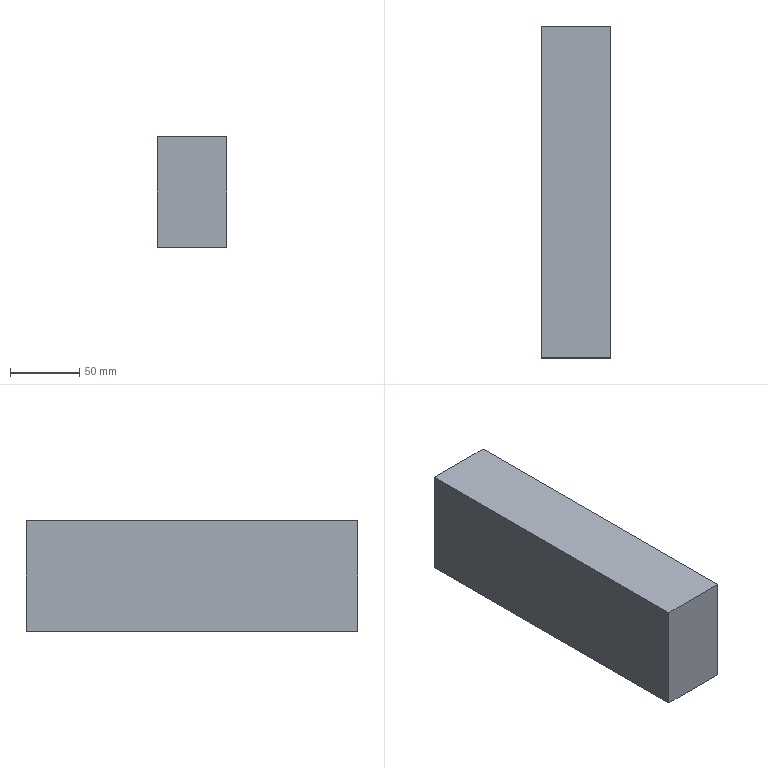Part | STEP file | Tube necking machine_id542_x_t | 1 solid | 6 faces | box 50 x 240 x 80 mm | volume 960000 mm3 | plane 6
STEP:
#1=CARTESIAN_POINT('',(0.,0.,0.));
#2=DIRECTION('',(0.,0.,1.));
#3=DIRECTION('',(1.,0.,0.));
#4=AXIS2_PLACEMENT_3D('',#1,#2,#3);
#5=CARTESIAN_POINT('',(160.,220.,0.));
#6=VERTEX_POINT('',#5);
#7=CARTESIAN_POINT('',(160.,-20.,0.));
#8=VERTEX_POINT('',#7);
#9=CARTESIAN_POINT('',(160.,220.,0.));
#10=DIRECTION('',(0.,-1.,0.));
#11=VECTOR('',#10,1.);
#12=LINE('',#9,#11);
#13=CARTESIAN_POINT('',(160.,220.,80.));
#14=DIRECTION('',(1.,0.,0.));
#15=DIRECTION('',(0.,1.,0.));
#16=AXIS2_PLACEMENT_3D('',#13,#14,#15);
#17=PLANE('',#16);
#18=CARTESIAN_POINT('',(0.,-80.));
#19=DIRECTION('',(-1.,0.));
#20=VECTOR('',#19,1.);
#21=LINE('',#18,#20);
#22=(GEOMETRIC_REPRESENTATION_CONTEXT(2)PARAMETRIC_REPRESENTATION_CONTEXT()REPRESENTATION_CONTEXT('',''));
#23=DEFINITIONAL_REPRESENTATION('',(#21),#22);
#24=PCURVE('',#17,#23);
#25=CARTESIAN_POINT('',(0.,0.,0.));
#26=DIRECTION('',(0.,0.,1.));
#27=DIRECTION('',(1.,0.,0.));
#28=AXIS2_PLACEMENT_3D('',#25,#26,#27);
#29=PLANE('',#28);
#30=CARTESIAN_POINT('',(160.,220.));
#31=DIRECTION('',(0.,-1.));
#32=VECTOR('',#31,1.);
#33=LINE('',#30,#32);
#34=(GEOMETRIC_REPRESENTATION_CONTEXT(2)PARAMETRIC_REPRESENTATION_CONTEXT()REPRESENTATION_CONTEXT('',''));
#35=DEFINITIONAL_REPRESENTATION('',(#33),#34);
#36=PCURVE('',#29,#35);
#37=SURFACE_CURVE('',#12,(#24,#36),.PCURVE_S1.);
#38=EDGE_CURVE('',#6,#8,#37,.T.);
#39=ORIENTED_EDGE('',*,*,#38,.T.);
#40=CARTESIAN_POINT('',(160.,-20.,80.));
#41=VERTEX_POINT('',#40);
#42=CARTESIAN_POINT('',(160.,-20.,80.));
#43=DIRECTION('',(0.,0.,-1.));
#44=VECTOR('',#43,1.);
#45=LINE('',#42,#44);
#46=CARTESIAN_POINT('',(-240.,0.));
#47=DIRECTION('',(0.,-1.));
#48=VECTOR('',#47,1.);
#49=LINE('',#46,#48);
#50=(GEOMETRIC_REPRESENTATION_CONTEXT(2)PARAMETRIC_REPRESENTATION_CONTEXT()REPRESENTATION_CONTEXT('',''));
#51=DEFINITIONAL_REPRESENTATION('',(#49),#50);
#52=PCURVE('',#17,#51);
#53=CARTESIAN_POINT('',(160.,-20.,80.));
#54=DIRECTION('',(0.,1.,0.));
#55=DIRECTION('',(-1.,0.,0.));
#56=AXIS2_PLACEMENT_3D('',#53,#54,#55);
#57=PLANE('',#56);
#58=CARTESIAN_POINT('',(0.,0.));
#59=DIRECTION('',(0.,-1.));
#60=VECTOR('',#59,1.);
#61=LINE('',#58,#60);
#62=(GEOMETRIC_REPRESENTATION_CONTEXT(2)PARAMETRIC_REPRESENTATION_CONTEXT()REPRESENTATION_CONTEXT('',''));
#63=DEFINITIONAL_REPRESENTATION('',(#61),#62);
#64=PCURVE('',#57,#63);
#65=SURFACE_CURVE('',#45,(#52,#64),.PCURVE_S1.);
#66=EDGE_CURVE('',#41,#8,#65,.T.);
#67=ORIENTED_EDGE('',*,*,#66,.F.);
#68=CARTESIAN_POINT('',(160.,220.,80.));
#69=VERTEX_POINT('',#68);
#70=CARTESIAN_POINT('',(160.,220.,80.));
#71=DIRECTION('',(0.,-1.,0.));
#72=VECTOR('',#71,1.);
#73=LINE('',#70,#72);
#74=CARTESIAN_POINT('',(0.,0.));
#75=DIRECTION('',(-1.,0.));
#76=VECTOR('',#75,1.);
#77=LINE('',#74,#76);
#78=(GEOMETRIC_REPRESENTATION_CONTEXT(2)PARAMETRIC_REPRESENTATION_CONTEXT()REPRESENTATION_CONTEXT('',''));
#79=DEFINITIONAL_REPRESENTATION('',(#77),#78);
#80=PCURVE('',#17,#79);
#81=CARTESIAN_POINT('',(0.,0.,80.));
#82=DIRECTION('',(0.,0.,1.));
#83=DIRECTION('',(1.,0.,0.));
#84=AXIS2_PLACEMENT_3D('',#81,#82,#83);
#85=PLANE('',#84);
#86=CARTESIAN_POINT('',(160.,220.));
#87=DIRECTION('',(0.,-1.));
#88=VECTOR('',#87,1.);
#89=LINE('',#86,#88);
#90=(GEOMETRIC_REPRESENTATION_CONTEXT(2)PARAMETRIC_REPRESENTATION_CONTEXT()REPRESENTATION_CONTEXT('',''));
#91=DEFINITIONAL_REPRESENTATION('',(#89),#90);
#92=PCURVE('',#85,#91);
#93=SURFACE_CURVE('',#73,(#80,#92),.PCURVE_S1.);
#94=EDGE_CURVE('',#69,#41,#93,.T.);
#95=ORIENTED_EDGE('',*,*,#94,.F.);
#96=CARTESIAN_POINT('',(160.,220.,80.));
#97=DIRECTION('',(0.,0.,-1.));
#98=VECTOR('',#97,1.);
#99=LINE('',#96,#98);
#100=CARTESIAN_POINT('',(0.,0.));
#101=DIRECTION('',(0.,-1.));
#102=VECTOR('',#101,1.);
#103=LINE('',#100,#102);
#104=(GEOMETRIC_REPRESENTATION_CONTEXT(2)PARAMETRIC_REPRESENTATION_CONTEXT()REPRESENTATION_CONTEXT('',''));
#105=DEFINITIONAL_REPRESENTATION('',(#103),#104);
#106=PCURVE('',#17,#105);
#107=CARTESIAN_POINT('',(210.,220.,80.));
#108=DIRECTION('',(0.,-1.,0.));
#109=DIRECTION('',(0.,0.,-1.));
#110=AXIS2_PLACEMENT_3D('',#107,#108,#109);
#111=PLANE('',#110);
#112=CARTESIAN_POINT('',(0.,-50.));
#113=DIRECTION('',(1.,0.));
#114=VECTOR('',#113,1.);
#115=LINE('',#112,#114);
#116=(GEOMETRIC_REPRESENTATION_CONTEXT(2)PARAMETRIC_REPRESENTATION_CONTEXT()REPRESENTATION_CONTEXT('',''));
#117=DEFINITIONAL_REPRESENTATION('',(#115),#116);
#118=PCURVE('',#111,#117);
#119=SURFACE_CURVE('',#99,(#106,#118),.PCURVE_S1.);
#120=EDGE_CURVE('',#69,#6,#119,.T.);
#121=ORIENTED_EDGE('',*,*,#120,.T.);
#122=EDGE_LOOP('',(#39,#67,#95,#121));
#123=FACE_BOUND('',#122,.T.);
#124=ADVANCED_FACE('',(#123),#17,.F.);
#125=CARTESIAN_POINT('',(210.,-20.,0.));
#126=VERTEX_POINT('',#125);
#127=CARTESIAN_POINT('',(160.,-20.,0.));
#128=DIRECTION('',(1.,0.,0.));
#129=VECTOR('',#128,1.);
#130=LINE('',#127,#129);
#131=CARTESIAN_POINT('',(0.,-80.));
#132=DIRECTION('',(-1.,0.));
#133=VECTOR('',#132,1.);
#134=LINE('',#131,#133);
#135=(GEOMETRIC_REPRESENTATION_CONTEXT(2)PARAMETRIC_REPRESENTATION_CONTEXT()REPRESENTATION_CONTEXT('',''));
#136=DEFINITIONAL_REPRESENTATION('',(#134),#135);
#137=PCURVE('',#57,#136);
#138=CARTESIAN_POINT('',(160.,-20.));
#139=DIRECTION('',(1.,0.));
#140=VECTOR('',#139,1.);
#141=LINE('',#138,#140);
#142=(GEOMETRIC_REPRESENTATION_CONTEXT(2)PARAMETRIC_REPRESENTATION_CONTEXT()REPRESENTATION_CONTEXT('',''));
#143=DEFINITIONAL_REPRESENTATION('',(#141),#142);
#144=PCURVE('',#29,#143);
#145=SURFACE_CURVE('',#130,(#137,#144),.PCURVE_S1.);
#146=EDGE_CURVE('',#8,#126,#145,.T.);
#147=ORIENTED_EDGE('',*,*,#146,.T.);
#148=CARTESIAN_POINT('',(210.,-20.,80.));
#149=VERTEX_POINT('',#148);
#150=CARTESIAN_POINT('',(210.,-20.,80.));
#151=DIRECTION('',(0.,0.,-1.));
#152=VECTOR('',#151,1.);
#153=LINE('',#150,#152);
#154=CARTESIAN_POINT('',(-50.,0.));
#155=DIRECTION('',(0.,-1.));
#156=VECTOR('',#155,1.);
#157=LINE('',#154,#156);
#158=(GEOMETRIC_REPRESENTATION_CONTEXT(2)PARAMETRIC_REPRESENTATION_CONTEXT()REPRESENTATION_CONTEXT('',''));
#159=DEFINITIONAL_REPRESENTATION('',(#157),#158);
#160=PCURVE('',#57,#159);
#161=CARTESIAN_POINT('',(210.,-20.,80.));
#162=DIRECTION('',(-1.,0.,0.));
#163=DIRECTION('',(0.,-1.,0.));
#164=AXIS2_PLACEMENT_3D('',#161,#162,#163);
#165=PLANE('',#164);
#166=CARTESIAN_POINT('',(0.,0.));
#167=DIRECTION('',(0.,-1.));
#168=VECTOR('',#167,1.);
#169=LINE('',#166,#168);
#170=(GEOMETRIC_REPRESENTATION_CONTEXT(2)PARAMETRIC_REPRESENTATION_CONTEXT()REPRESENTATION_CONTEXT('',''));
#171=DEFINITIONAL_REPRESENTATION('',(#169),#170);
#172=PCURVE('',#165,#171);
#173=SURFACE_CURVE('',#153,(#160,#172),.PCURVE_S1.);
#174=EDGE_CURVE('',#149,#126,#173,.T.);
#175=ORIENTED_EDGE('',*,*,#174,.F.);
#176=CARTESIAN_POINT('',(160.,-20.,80.));
#177=DIRECTION('',(1.,0.,0.));
#178=VECTOR('',#177,1.);
#179=LINE('',#176,#178);
#180=CARTESIAN_POINT('',(0.,0.));
#181=DIRECTION('',(-1.,0.));
#182=VECTOR('',#181,1.);
#183=LINE('',#180,#182);
#184=(GEOMETRIC_REPRESENTATION_CONTEXT(2)PARAMETRIC_REPRESENTATION_CONTEXT()REPRESENTATION_CONTEXT('',''));
#185=DEFINITIONAL_REPRESENTATION('',(#183),#184);
#186=PCURVE('',#57,#185);
#187=CARTESIAN_POINT('',(160.,-20.));
#188=DIRECTION('',(1.,0.));
#189=VECTOR('',#188,1.);
#190=LINE('',#187,#189);
#191=(GEOMETRIC_REPRESENTATION_CONTEXT(2)PARAMETRIC_REPRESENTATION_CONTEXT()REPRESENTATION_CONTEXT('',''));
#192=DEFINITIONAL_REPRESENTATION('',(#190),#191);
#193=PCURVE('',#85,#192);
#194=SURFACE_CURVE('',#179,(#186,#193),.PCURVE_S1.);
#195=EDGE_CURVE('',#41,#149,#194,.T.);
#196=ORIENTED_EDGE('',*,*,#195,.F.);
#197=ORIENTED_EDGE('',*,*,#66,.T.);
#198=EDGE_LOOP('',(#147,#175,#196,#197));
#199=FACE_BOUND('',#198,.T.);
#200=ADVANCED_FACE('',(#199),#57,.F.);
#201=CARTESIAN_POINT('',(210.,220.,0.));
#202=VERTEX_POINT('',#201);
#203=CARTESIAN_POINT('',(210.,-20.,0.));
#204=DIRECTION('',(0.,1.,0.));
#205=VECTOR('',#204,1.);
#206=LINE('',#203,#205);
#207=CARTESIAN_POINT('',(0.,-80.));
#208=DIRECTION('',(-1.,0.));
#209=VECTOR('',#208,1.);
#210=LINE('',#207,#209);
#211=(GEOMETRIC_REPRESENTATION_CONTEXT(2)PARAMETRIC_REPRESENTATION_CONTEXT()REPRESENTATION_CONTEXT('',''));
#212=DEFINITIONAL_REPRESENTATION('',(#210),#211);
#213=PCURVE('',#165,#212);
#214=CARTESIAN_POINT('',(210.,-20.));
#215=DIRECTION('',(0.,1.));
#216=VECTOR('',#215,1.);
#217=LINE('',#214,#216);
#218=(GEOMETRIC_REPRESENTATION_CONTEXT(2)PARAMETRIC_REPRESENTATION_CONTEXT()REPRESENTATION_CONTEXT('',''));
#219=DEFINITIONAL_REPRESENTATION('',(#217),#218);
#220=PCURVE('',#29,#219);
#221=SURFACE_CURVE('',#206,(#213,#220),.PCURVE_S1.);
#222=EDGE_CURVE('',#126,#202,#221,.T.);
#223=ORIENTED_EDGE('',*,*,#222,.T.);
#224=CARTESIAN_POINT('',(210.,220.,80.));
#225=VERTEX_POINT('',#224);
#226=CARTESIAN_POINT('',(210.,220.,80.));
#227=DIRECTION('',(0.,0.,-1.));
#228=VECTOR('',#227,1.);
#229=LINE('',#226,#228);
#230=CARTESIAN_POINT('',(-240.,0.));
#231=DIRECTION('',(0.,-1.));
#232=VECTOR('',#231,1.);
#233=LINE('',#230,#232);
#234=(GEOMETRIC_REPRESENTATION_CONTEXT(2)PARAMETRIC_REPRESENTATION_CONTEXT()REPRESENTATION_CONTEXT('',''));
#235=DEFINITIONAL_REPRESENTATION('',(#233),#234);
#236=PCURVE('',#165,#235);
#237=CARTESIAN_POINT('',(0.,0.));
#238=DIRECTION('',(1.,0.));
#239=VECTOR('',#238,1.);
#240=LINE('',#237,#239);
#241=(GEOMETRIC_REPRESENTATION_CONTEXT(2)PARAMETRIC_REPRESENTATION_CONTEXT()REPRESENTATION_CONTEXT('',''));
#242=DEFINITIONAL_REPRESENTATION('',(#240),#241);
#243=PCURVE('',#111,#242);
#244=SURFACE_CURVE('',#229,(#236,#243),.PCURVE_S1.);
#245=EDGE_CURVE('',#225,#202,#244,.T.);
#246=ORIENTED_EDGE('',*,*,#245,.F.);
#247=CARTESIAN_POINT('',(210.,-20.,80.));
#248=DIRECTION('',(0.,1.,0.));
#249=VECTOR('',#248,1.);
#250=LINE('',#247,#249);
#251=CARTESIAN_POINT('',(0.,0.));
#252=DIRECTION('',(-1.,0.));
#253=VECTOR('',#252,1.);
#254=LINE('',#251,#253);
#255=(GEOMETRIC_REPRESENTATION_CONTEXT(2)PARAMETRIC_REPRESENTATION_CONTEXT()REPRESENTATION_CONTEXT('',''));
#256=DEFINITIONAL_REPRESENTATION('',(#254),#255);
#257=PCURVE('',#165,#256);
#258=CARTESIAN_POINT('',(210.,-20.));
#259=DIRECTION('',(0.,1.));
#260=VECTOR('',#259,1.);
#261=LINE('',#258,#260);
#262=(GEOMETRIC_REPRESENTATION_CONTEXT(2)PARAMETRIC_REPRESENTATION_CONTEXT()REPRESENTATION_CONTEXT('',''));
#263=DEFINITIONAL_REPRESENTATION('',(#261),#262);
#264=PCURVE('',#85,#263);
#265=SURFACE_CURVE('',#250,(#257,#264),.PCURVE_S1.);
#266=EDGE_CURVE('',#149,#225,#265,.T.);
#267=ORIENTED_EDGE('',*,*,#266,.F.);
#268=ORIENTED_EDGE('',*,*,#174,.T.);
#269=EDGE_LOOP('',(#223,#246,#267,#268));
#270=FACE_BOUND('',#269,.T.);
#271=ADVANCED_FACE('',(#270),#165,.F.);
#272=CARTESIAN_POINT('',(210.,220.,0.));
#273=DIRECTION('',(-1.,0.,0.));
#274=VECTOR('',#273,1.);
#275=LINE('',#272,#274);
#276=CARTESIAN_POINT('',(80.,0.));
#277=DIRECTION('',(0.,-1.));
#278=VECTOR('',#277,1.);
#279=LINE('',#276,#278);
#280=(GEOMETRIC_REPRESENTATION_CONTEXT(2)PARAMETRIC_REPRESENTATION_CONTEXT()REPRESENTATION_CONTEXT('',''));
#281=DEFINITIONAL_REPRESENTATION('',(#279),#280);
#282=PCURVE('',#111,#281);
#283=CARTESIAN_POINT('',(210.,220.));
#284=DIRECTION('',(-1.,0.));
#285=VECTOR('',#284,1.);
#286=LINE('',#283,#285);
#287=(GEOMETRIC_REPRESENTATION_CONTEXT(2)PARAMETRIC_REPRESENTATION_CONTEXT()REPRESENTATION_CONTEXT('',''));
#288=DEFINITIONAL_REPRESENTATION('',(#286),#287);
#289=PCURVE('',#29,#288);
#290=SURFACE_CURVE('',#275,(#282,#289),.PCURVE_S1.);
#291=EDGE_CURVE('',#202,#6,#290,.T.);
#292=ORIENTED_EDGE('',*,*,#291,.T.);
#293=ORIENTED_EDGE('',*,*,#120,.F.);
#294=CARTESIAN_POINT('',(210.,220.,80.));
#295=DIRECTION('',(-1.,0.,0.));
#296=VECTOR('',#295,1.);
#297=LINE('',#294,#296);
#298=CARTESIAN_POINT('',(0.,0.));
#299=DIRECTION('',(0.,-1.));
#300=VECTOR('',#299,1.);
#301=LINE('',#298,#300);
#302=(GEOMETRIC_REPRESENTATION_CONTEXT(2)PARAMETRIC_REPRESENTATION_CONTEXT()REPRESENTATION_CONTEXT('',''));
#303=DEFINITIONAL_REPRESENTATION('',(#301),#302);
#304=PCURVE('',#111,#303);
#305=CARTESIAN_POINT('',(210.,220.));
#306=DIRECTION('',(-1.,0.));
#307=VECTOR('',#306,1.);
#308=LINE('',#305,#307);
#309=(GEOMETRIC_REPRESENTATION_CONTEXT(2)PARAMETRIC_REPRESENTATION_CONTEXT()REPRESENTATION_CONTEXT('',''));
#310=DEFINITIONAL_REPRESENTATION('',(#308),#309);
#311=PCURVE('',#85,#310);
#312=SURFACE_CURVE('',#297,(#304,#311),.PCURVE_S1.);
#313=EDGE_CURVE('',#225,#69,#312,.T.);
#314=ORIENTED_EDGE('',*,*,#313,.F.);
#315=ORIENTED_EDGE('',*,*,#245,.T.);
#316=EDGE_LOOP('',(#292,#293,#314,#315));
#317=FACE_BOUND('',#316,.T.);
#318=ADVANCED_FACE('',(#317),#111,.F.);
#319=ORIENTED_EDGE('',*,*,#94,.T.);
#320=ORIENTED_EDGE('',*,*,#195,.T.);
#321=ORIENTED_EDGE('',*,*,#266,.T.);
#322=ORIENTED_EDGE('',*,*,#313,.T.);
#323=EDGE_LOOP('',(#319,#320,#321,#322));
#324=FACE_BOUND('',#323,.T.);
#325=ADVANCED_FACE('',(#324),#85,.T.);
#326=ORIENTED_EDGE('',*,*,#38,.F.);
#327=ORIENTED_EDGE('',*,*,#291,.F.);
#328=ORIENTED_EDGE('',*,*,#222,.F.);
#329=ORIENTED_EDGE('',*,*,#146,.F.);
#330=EDGE_LOOP('',(#326,#327,#328,#329));
#331=FACE_BOUND('',#330,.T.);
#332=ADVANCED_FACE('',(#331),#29,.F.);
#333=CLOSED_SHELL('',(#124,#200,#271,#318,#325,#332));
#334=MANIFOLD_SOLID_BREP('',#333);
#335=(LENGTH_UNIT()NAMED_UNIT(*)SI_UNIT(.MILLI.,.METRE.));
#336=UNCERTAINTY_MEASURE_WITH_UNIT(LENGTH_MEASURE(0.0000001),#335,'','');
#337=(NAMED_UNIT(*)PLANE_ANGLE_UNIT()SI_UNIT($,.RADIAN.));
#338=(NAMED_UNIT(*)SI_UNIT($,.STERADIAN.)SOLID_ANGLE_UNIT());
#339=(GEOMETRIC_REPRESENTATION_CONTEXT(3)GLOBAL_UNCERTAINTY_ASSIGNED_CONTEXT((#336))GLOBAL_UNIT_ASSIGNED_CONTEXT((#335,#337,#338))REPRESENTATION_CONTEXT('',''));
#340=ADVANCED_BREP_SHAPE_REPRESENTATION('',(#4,#334),#339);